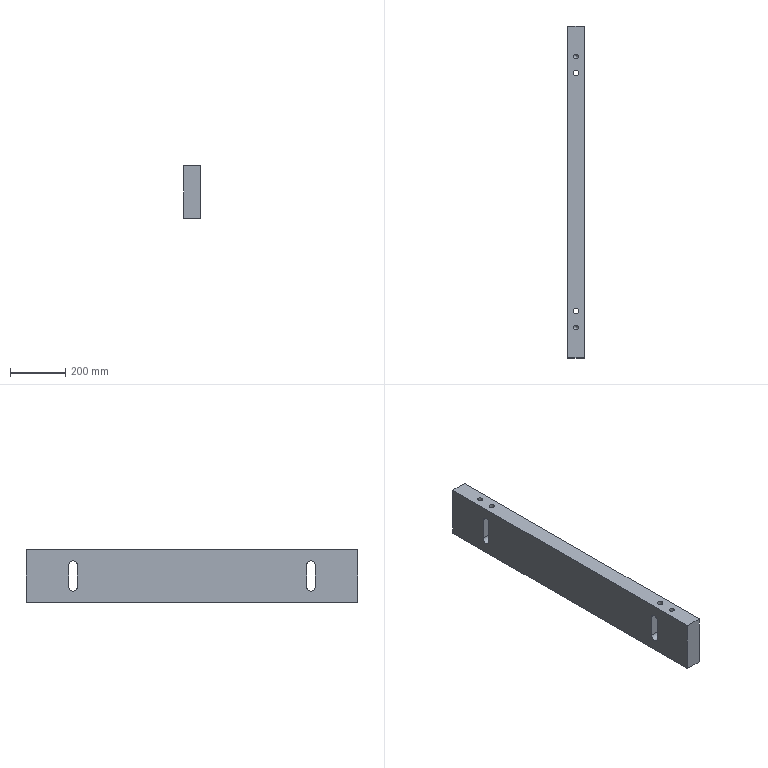Part | STEP file | lll_id4454_x_t | 1 solid | 30 faces | box 60 x 1200 x 190 mm | volume 13210878 mm3 | cylinder 14 | plane 10 | cone 6 | commonest cylinder face diameters 20 x4 30 x4 6.806 x2 17.505 x2 17.506 x2
STEP:
#1=CARTESIAN_POINT('',(207.435,-430.,-220.));
#2=VERTEX_POINT('',#1);
#3=CARTESIAN_POINT('',(207.435,-427.265,-220.));
#4=CARTESIAN_POINT('',(207.435,-432.735,-220.));
#5=CARTESIAN_POINT('',(206.282,-435.303,-220.824));
#6=CARTESIAN_POINT('',(203.596,-437.978,-222.257));
#7=CARTESIAN_POINT('',(202.537,-438.697,-222.762));
#8=CARTESIAN_POINT('',(200.161,-439.708,-223.547));
#9=CARTESIAN_POINT('',(198.811,-439.997,-223.817));
#10=CARTESIAN_POINT('',(194.742,-440.005,-223.824));
#11=CARTESIAN_POINT('',(192.2,-438.892,-222.75));
#12=CARTESIAN_POINT('',(189.491,-436.205,-221.306));
#13=CARTESIAN_POINT('',(188.758,-435.142,-220.853));
#14=CARTESIAN_POINT('',(187.723,-432.721,-220.196));
#15=CARTESIAN_POINT('',(187.438,-431.369,-220.002));
#16=CARTESIAN_POINT('',(187.432,-428.674,-219.998));
#17=CARTESIAN_POINT('',(187.71,-427.321,-220.187));
#18=CARTESIAN_POINT('',(188.743,-424.881,-220.844));
#19=CARTESIAN_POINT('',(189.483,-423.806,-221.301));
#20=CARTESIAN_POINT('',(192.176,-421.125,-222.738));
#21=CARTESIAN_POINT('',(194.698,-420.001,-223.819));
#22=CARTESIAN_POINT('',(200.165,-419.999,-223.821));
#23=CARTESIAN_POINT('',(202.693,-421.126,-222.738));
#24=CARTESIAN_POINT('',(206.281,-424.694,-220.824));
#25=CARTESIAN_POINT('',(207.435,-427.265,-220.));
#26=CARTESIAN_POINT('',(207.435,-432.735,-220.));
#27=B_SPLINE_CURVE_WITH_KNOTS('',3,(#3,#4,#5,#6,#7,#8,#9,#10,#11,#12,#13,#14,#15,#16,#17,#18,#19,#20,#21,#22,#23,#24,#25,#26),.UNSPECIFIED.,.T.,.F.,(2,2,2,2,2,2,2,2,2,2,2,2,2,2),(-0.125,0.,0.125,0.1875,0.25,0.375,0.4375,0.5,0.5625,0.625,0.75,0.875,1.,1.125),.UNSPECIFIED.);
#28=EDGE_CURVE('',#2,#2,#27,.T.);
#29=ORIENTED_EDGE('',*,*,#28,.T.);
#30=EDGE_LOOP('',(#29));
#31=FACE_BOUND('',#30,.T.);
#32=CARTESIAN_POINT('',(187.435,-430.,-180.));
#33=VERTEX_POINT('',#32);
#34=CARTESIAN_POINT('',(197.435,-430.,-180.));
#35=DIRECTION('',(0.,0.,-1.));
#36=DIRECTION('',(-1.,0.,0.));
#37=AXIS2_PLACEMENT_3D('',#34,#35,#36);
#38=CIRCLE('',#37,10.);
#39=EDGE_CURVE('',#33,#33,#38,.T.);
#40=ORIENTED_EDGE('',*,*,#39,.F.);
#41=EDGE_LOOP('',(#40));
#42=FACE_BOUND('',#41,.T.);
#43=CARTESIAN_POINT('',(197.435,-430.,-80.));
#44=DIRECTION('',(0.,0.,-1.));
#45=DIRECTION('',(-1.,0.,0.));
#46=AXIS2_PLACEMENT_3D('',#43,#44,#45);
#47=CYLINDRICAL_SURFACE('',#46,10.);
#48=ADVANCED_FACE('',(#31,#42),#47,.F.);
#49=CARTESIAN_POINT('',(207.435,430.,-220.));
#50=VERTEX_POINT('',#49);
#51=CARTESIAN_POINT('',(207.435,432.735,-220.));
#52=CARTESIAN_POINT('',(207.435,427.265,-220.));
#53=CARTESIAN_POINT('',(206.282,424.697,-220.824));
#54=CARTESIAN_POINT('',(203.596,422.022,-222.257));
#55=CARTESIAN_POINT('',(202.537,421.303,-222.762));
#56=CARTESIAN_POINT('',(200.161,420.292,-223.547));
#57=CARTESIAN_POINT('',(198.811,420.003,-223.817));
#58=CARTESIAN_POINT('',(194.742,419.995,-223.824));
#59=CARTESIAN_POINT('',(192.2,421.108,-222.75));
#60=CARTESIAN_POINT('',(189.491,423.795,-221.306));
#61=CARTESIAN_POINT('',(188.758,424.858,-220.853));
#62=CARTESIAN_POINT('',(187.723,427.279,-220.196));
#63=CARTESIAN_POINT('',(187.438,428.631,-220.002));
#64=CARTESIAN_POINT('',(187.432,431.326,-219.998));
#65=CARTESIAN_POINT('',(187.71,432.679,-220.187));
#66=CARTESIAN_POINT('',(188.743,435.119,-220.844));
#67=CARTESIAN_POINT('',(189.483,436.194,-221.301));
#68=CARTESIAN_POINT('',(192.176,438.875,-222.738));
#69=CARTESIAN_POINT('',(194.698,439.999,-223.819));
#70=CARTESIAN_POINT('',(200.165,440.001,-223.821));
#71=CARTESIAN_POINT('',(202.693,438.874,-222.738));
#72=CARTESIAN_POINT('',(206.281,435.306,-220.824));
#73=CARTESIAN_POINT('',(207.435,432.735,-220.));
#74=CARTESIAN_POINT('',(207.435,427.265,-220.));
#75=B_SPLINE_CURVE_WITH_KNOTS('',3,(#51,#52,#53,#54,#55,#56,#57,#58,#59,#60,#61,#62,#63,#64,#65,#66,#67,#68,#69,#70,#71,#72,#73,#74),.UNSPECIFIED.,.T.,.F.,(2,2,2,2,2,2,2,2,2,2,2,2,2,2),(-0.125,0.,0.125,0.1875,0.25,0.375,0.4375,0.5,0.5625,0.625,0.75,0.875,1.,1.125),.UNSPECIFIED.);
#76=EDGE_CURVE('',#50,#50,#75,.T.);
#77=ORIENTED_EDGE('',*,*,#76,.T.);
#78=EDGE_LOOP('',(#77));
#79=FACE_BOUND('',#78,.T.);
#80=CARTESIAN_POINT('',(187.435,430.,-180.));
#81=VERTEX_POINT('',#80);
#82=CARTESIAN_POINT('',(197.435,430.,-180.));
#83=DIRECTION('',(0.,0.,-1.));
#84=DIRECTION('',(-1.,0.,0.));
#85=AXIS2_PLACEMENT_3D('',#82,#83,#84);
#86=CIRCLE('',#85,10.);
#87=EDGE_CURVE('',#81,#81,#86,.T.);
#88=ORIENTED_EDGE('',*,*,#87,.F.);
#89=EDGE_LOOP('',(#88));
#90=FACE_BOUND('',#89,.T.);
#91=CARTESIAN_POINT('',(197.435,430.,-80.));
#92=DIRECTION('',(0.,0.,-1.));
#93=DIRECTION('',(-1.,0.,0.));
#94=AXIS2_PLACEMENT_3D('',#91,#92,#93);
#95=CYLINDRICAL_SURFACE('',#94,10.);
#96=ADVANCED_FACE('',(#79,#90),#95,.F.);
#97=CARTESIAN_POINT('',(227.435,-445.,-235.));
#98=VERTEX_POINT('',#97);
#99=CARTESIAN_POINT('',(227.435,-445.,-315.));
#100=VERTEX_POINT('',#99);
#101=CARTESIAN_POINT('',(227.435,-445.,-182.5));
#102=DIRECTION('',(0.,0.,-1.));
#103=VECTOR('',#102,1.);
#104=LINE('',#101,#103);
#105=EDGE_CURVE('',#98,#100,#104,.T.);
#106=ORIENTED_EDGE('',*,*,#105,.F.);
#107=CARTESIAN_POINT('',(227.435,-415.,-235.));
#108=VERTEX_POINT('',#107);
#109=CARTESIAN_POINT('',(227.435,-430.,-235.));
#110=DIRECTION('',(1.,0.,0.));
#111=DIRECTION('',(0.,0.,-1.));
#112=AXIS2_PLACEMENT_3D('',#109,#110,#111);
#113=CIRCLE('',#112,15.);
#114=EDGE_CURVE('',#108,#98,#113,.T.);
#115=ORIENTED_EDGE('',*,*,#114,.F.);
#116=CARTESIAN_POINT('',(227.435,-415.,-315.));
#117=VERTEX_POINT('',#116);
#118=CARTESIAN_POINT('',(227.435,-415.,-182.5));
#119=DIRECTION('',(0.,0.,1.));
#120=VECTOR('',#119,1.);
#121=LINE('',#118,#120);
#122=EDGE_CURVE('',#117,#108,#121,.T.);
#123=ORIENTED_EDGE('',*,*,#122,.F.);
#124=CARTESIAN_POINT('',(227.435,-430.,-315.));
#125=DIRECTION('',(1.,0.,0.));
#126=DIRECTION('',(0.,0.,-1.));
#127=AXIS2_PLACEMENT_3D('',#124,#125,#126);
#128=CIRCLE('',#127,15.);
#129=EDGE_CURVE('',#100,#117,#128,.T.);
#130=ORIENTED_EDGE('',*,*,#129,.F.);
#131=EDGE_LOOP('',(#106,#115,#123,#130));
#132=FACE_BOUND('',#131,.T.);
#133=CARTESIAN_POINT('',(227.435,415.,-235.));
#134=VERTEX_POINT('',#133);
#135=CARTESIAN_POINT('',(227.435,415.,-315.));
#136=VERTEX_POINT('',#135);
#137=CARTESIAN_POINT('',(227.435,415.,-182.5));
#138=DIRECTION('',(0.,0.,-1.));
#139=VECTOR('',#138,1.);
#140=LINE('',#137,#139);
#141=EDGE_CURVE('',#134,#136,#140,.T.);
#142=ORIENTED_EDGE('',*,*,#141,.F.);
#143=CARTESIAN_POINT('',(227.435,445.,-235.));
#144=VERTEX_POINT('',#143);
#145=CARTESIAN_POINT('',(227.435,430.,-235.));
#146=DIRECTION('',(1.,0.,0.));
#147=DIRECTION('',(0.,0.,-1.));
#148=AXIS2_PLACEMENT_3D('',#145,#146,#147);
#149=CIRCLE('',#148,15.);
#150=EDGE_CURVE('',#144,#134,#149,.T.);
#151=ORIENTED_EDGE('',*,*,#150,.F.);
#152=CARTESIAN_POINT('',(227.435,445.,-315.));
#153=VERTEX_POINT('',#152);
#154=CARTESIAN_POINT('',(227.435,445.,-182.5));
#155=DIRECTION('',(0.,0.,1.));
#156=VECTOR('',#155,1.);
#157=LINE('',#154,#156);
#158=EDGE_CURVE('',#153,#144,#157,.T.);
#159=ORIENTED_EDGE('',*,*,#158,.F.);
#160=CARTESIAN_POINT('',(227.435,430.,-315.));
#161=DIRECTION('',(1.,0.,0.));
#162=DIRECTION('',(0.,0.,-1.));
#163=AXIS2_PLACEMENT_3D('',#160,#161,#162);
#164=CIRCLE('',#163,15.);
#165=EDGE_CURVE('',#136,#153,#164,.T.);
#166=ORIENTED_EDGE('',*,*,#165,.F.);
#167=EDGE_LOOP('',(#142,#151,#159,#166));
#168=FACE_BOUND('',#167,.T.);
#169=CARTESIAN_POINT('',(227.435,109.597,-194.345));
#170=VERTEX_POINT('',#169);
#171=CARTESIAN_POINT('',(227.435,113.,-194.345));
#172=DIRECTION('',(-1.,0.,0.));
#173=DIRECTION('',(0.,-1.,0.));
#174=AXIS2_PLACEMENT_3D('',#171,#172,#173);
#175=CIRCLE('',#174,3.403);
#176=EDGE_CURVE('',#170,#170,#175,.T.);
#177=ORIENTED_EDGE('',*,*,#176,.T.);
#178=EDGE_LOOP('',(#177));
#179=FACE_BOUND('',#178,.T.);
#180=CARTESIAN_POINT('',(227.435,-600.,-180.));
#181=VERTEX_POINT('',#180);
#182=CARTESIAN_POINT('',(227.435,-600.,-370.));
#183=VERTEX_POINT('',#182);
#184=CARTESIAN_POINT('',(227.435,-600.,-182.5));
#185=DIRECTION('',(0.,0.,-1.));
#186=VECTOR('',#185,1.);
#187=LINE('',#184,#186);
#188=EDGE_CURVE('',#181,#183,#187,.T.);
#189=ORIENTED_EDGE('',*,*,#188,.T.);
#190=CARTESIAN_POINT('',(227.435,600.,-370.));
#191=VERTEX_POINT('',#190);
#192=CARTESIAN_POINT('',(227.435,600.,-370.));
#193=DIRECTION('',(0.,-1.,0.));
#194=VECTOR('',#193,1.);
#195=LINE('',#192,#194);
#196=EDGE_CURVE('',#191,#183,#195,.T.);
#197=ORIENTED_EDGE('',*,*,#196,.F.);
#198=CARTESIAN_POINT('',(227.435,600.,-180.));
#199=VERTEX_POINT('',#198);
#200=CARTESIAN_POINT('',(227.435,600.,-182.5));
#201=DIRECTION('',(0.,0.,-1.));
#202=VECTOR('',#201,1.);
#203=LINE('',#200,#202);
#204=EDGE_CURVE('',#199,#191,#203,.T.);
#205=ORIENTED_EDGE('',*,*,#204,.F.);
#206=CARTESIAN_POINT('',(227.435,1.,-180.));
#207=DIRECTION('',(0.,-1.,0.));
#208=VECTOR('',#207,1.);
#209=LINE('',#206,#208);
#210=EDGE_CURVE('',#199,#181,#209,.T.);
#211=ORIENTED_EDGE('',*,*,#210,.T.);
#212=EDGE_LOOP('',(#189,#197,#205,#211));
#213=FACE_BOUND('',#212,.T.);
#214=CARTESIAN_POINT('',(227.435,-206.403,-194.345));
#215=VERTEX_POINT('',#214);
#216=CARTESIAN_POINT('',(227.435,-203.,-194.345));
#217=DIRECTION('',(-1.,0.,0.));
#218=DIRECTION('',(0.,-1.,0.));
#219=AXIS2_PLACEMENT_3D('',#216,#217,#218);
#220=CIRCLE('',#219,3.403);
#221=EDGE_CURVE('',#215,#215,#220,.T.);
#222=ORIENTED_EDGE('',*,*,#221,.T.);
#223=EDGE_LOOP('',(#222));
#224=FACE_BOUND('',#223,.T.);
#225=CARTESIAN_POINT('',(227.435,600.,-182.5));
#226=DIRECTION('',(1.,0.,0.));
#227=DIRECTION('',(0.,0.,-1.));
#228=AXIS2_PLACEMENT_3D('',#225,#226,#227);
#229=PLANE('',#228);
#230=ADVANCED_FACE('',(#132,#168,#179,#213,#224),#229,.T.);
#231=CARTESIAN_POINT('',(187.435,430.,-370.));
#232=VERTEX_POINT('',#231);
#233=CARTESIAN_POINT('',(197.435,430.,-370.));
#234=DIRECTION('',(0.,0.,-1.));
#235=DIRECTION('',(-1.,0.,0.));
#236=AXIS2_PLACEMENT_3D('',#233,#234,#235);
#237=CIRCLE('',#236,10.);
#238=EDGE_CURVE('',#232,#232,#237,.T.);
#239=ORIENTED_EDGE('',*,*,#238,.F.);
#240=EDGE_LOOP('',(#239));
#241=FACE_BOUND('',#240,.T.);
#242=CARTESIAN_POINT('',(187.435,-430.,-370.));
#243=VERTEX_POINT('',#242);
#244=CARTESIAN_POINT('',(197.435,-430.,-370.));
#245=DIRECTION('',(0.,0.,-1.));
#246=DIRECTION('',(-1.,0.,0.));
#247=AXIS2_PLACEMENT_3D('',#244,#245,#246);
#248=CIRCLE('',#247,10.);
#249=EDGE_CURVE('',#243,#243,#248,.T.);
#250=ORIENTED_EDGE('',*,*,#249,.F.);
#251=EDGE_LOOP('',(#250));
#252=FACE_BOUND('',#251,.T.);
#253=CARTESIAN_POINT('',(206.188,-490.,-370.));
#254=VERTEX_POINT('',#253);
#255=CARTESIAN_POINT('',(197.435,-490.,-370.));
#256=DIRECTION('',(0.,0.,1.));
#257=DIRECTION('',(1.,0.,0.));
#258=AXIS2_PLACEMENT_3D('',#255,#256,#257);
#259=CIRCLE('',#258,8.752);
#260=EDGE_CURVE('',#254,#254,#259,.T.);
#261=ORIENTED_EDGE('',*,*,#260,.T.);
#262=EDGE_LOOP('',(#261));
#263=FACE_BOUND('',#262,.T.);
#264=ORIENTED_EDGE('',*,*,#196,.T.);
#265=CARTESIAN_POINT('',(167.435,-600.,-370.));
#266=VERTEX_POINT('',#265);
#267=CARTESIAN_POINT('',(227.435,-600.,-370.));
#268=DIRECTION('',(-1.,0.,0.));
#269=VECTOR('',#268,1.);
#270=LINE('',#267,#269);
#271=EDGE_CURVE('',#183,#266,#270,.T.);
#272=ORIENTED_EDGE('',*,*,#271,.T.);
#273=CARTESIAN_POINT('',(167.435,600.,-370.));
#274=VERTEX_POINT('',#273);
#275=CARTESIAN_POINT('',(167.435,1.,-370.));
#276=DIRECTION('',(0.,-1.,0.));
#277=VECTOR('',#276,1.);
#278=LINE('',#275,#277);
#279=EDGE_CURVE('',#274,#266,#278,.T.);
#280=ORIENTED_EDGE('',*,*,#279,.F.);
#281=CARTESIAN_POINT('',(-3742.565,600.,-370.));
#282=DIRECTION('',(1.,0.,0.));
#283=VECTOR('',#282,1.);
#284=LINE('',#281,#283);
#285=EDGE_CURVE('',#274,#191,#284,.T.);
#286=ORIENTED_EDGE('',*,*,#285,.T.);
#287=EDGE_LOOP('',(#264,#272,#280,#286));
#288=FACE_BOUND('',#287,.T.);
#289=CARTESIAN_POINT('',(206.188,490.,-370.));
#290=VERTEX_POINT('',#289);
#291=CARTESIAN_POINT('',(197.435,490.,-370.));
#292=DIRECTION('',(0.,0.,1.));
#293=DIRECTION('',(1.,0.,0.));
#294=AXIS2_PLACEMENT_3D('',#291,#292,#293);
#295=CIRCLE('',#294,8.752);
#296=EDGE_CURVE('',#290,#290,#295,.T.);
#297=ORIENTED_EDGE('',*,*,#296,.T.);
#298=EDGE_LOOP('',(#297));
#299=FACE_BOUND('',#298,.T.);
#300=CARTESIAN_POINT('',(2413.751,1.,-370.));
#301=DIRECTION('',(0.,0.,-1.));
#302=DIRECTION('',(-1.,0.,0.));
#303=AXIS2_PLACEMENT_3D('',#300,#301,#302);
#304=PLANE('',#303);
#305=ADVANCED_FACE('',(#241,#252,#263,#288,#299),#304,.T.);
#306=ORIENTED_EDGE('',*,*,#39,.T.);
#307=EDGE_LOOP('',(#306));
#308=FACE_BOUND('',#307,.T.);
#309=ORIENTED_EDGE('',*,*,#87,.T.);
#310=EDGE_LOOP('',(#309));
#311=FACE_BOUND('',#310,.T.);
#312=CARTESIAN_POINT('',(188.682,490.,-180.));
#313=VERTEX_POINT('',#312);
#314=CARTESIAN_POINT('',(197.435,490.,-180.));
#315=DIRECTION('',(0.,0.,-1.));
#316=DIRECTION('',(-1.,0.,0.));
#317=AXIS2_PLACEMENT_3D('',#314,#315,#316);
#318=CIRCLE('',#317,8.753);
#319=EDGE_CURVE('',#313,#313,#318,.T.);
#320=ORIENTED_EDGE('',*,*,#319,.T.);
#321=EDGE_LOOP('',(#320));
#322=FACE_BOUND('',#321,.T.);
#323=CARTESIAN_POINT('',(188.682,-490.,-180.));
#324=VERTEX_POINT('',#323);
#325=CARTESIAN_POINT('',(197.435,-490.,-180.));
#326=DIRECTION('',(0.,0.,-1.));
#327=DIRECTION('',(-1.,0.,0.));
#328=AXIS2_PLACEMENT_3D('',#325,#326,#327);
#329=CIRCLE('',#328,8.753);
#330=EDGE_CURVE('',#324,#324,#329,.T.);
#331=ORIENTED_EDGE('',*,*,#330,.T.);
#332=EDGE_LOOP('',(#331));
#333=FACE_BOUND('',#332,.T.);
#334=CARTESIAN_POINT('',(167.435,-600.,-180.));
#335=VERTEX_POINT('',#334);
#336=CARTESIAN_POINT('',(2413.751,-600.,-180.));
#337=DIRECTION('',(-1.,0.,0.));
#338=VECTOR('',#337,1.);
#339=LINE('',#336,#338);
#340=EDGE_CURVE('',#181,#335,#339,.T.);
#341=ORIENTED_EDGE('',*,*,#340,.F.);
#342=ORIENTED_EDGE('',*,*,#210,.F.);
#343=CARTESIAN_POINT('',(167.435,600.,-180.));
#344=VERTEX_POINT('',#343);
#345=CARTESIAN_POINT('',(2413.751,600.,-180.));
#346=DIRECTION('',(1.,0.,0.));
#347=VECTOR('',#346,1.);
#348=LINE('',#345,#347);
#349=EDGE_CURVE('',#344,#199,#348,.T.);
#350=ORIENTED_EDGE('',*,*,#349,.F.);
#351=CARTESIAN_POINT('',(167.435,0.,-180.));
#352=DIRECTION('',(0.,1.,0.));
#353=VECTOR('',#352,1.);
#354=LINE('',#351,#353);
#355=EDGE_CURVE('',#335,#344,#354,.T.);
#356=ORIENTED_EDGE('',*,*,#355,.F.);
#357=EDGE_LOOP('',(#341,#342,#350,#356));
#358=FACE_BOUND('',#357,.T.);
#359=CARTESIAN_POINT('',(2413.751,1.,-180.));
#360=DIRECTION('',(0.,0.,-1.));
#361=DIRECTION('',(-1.,0.,0.));
#362=AXIS2_PLACEMENT_3D('',#359,#360,#361);
#363=PLANE('',#362);
#364=ADVANCED_FACE('',(#308,#311,#322,#333,#358),#363,.F.);
#365=CARTESIAN_POINT('',(167.435,-600.,-182.5));
#366=DIRECTION('',(0.,0.,-1.));
#367=VECTOR('',#366,1.);
#368=LINE('',#365,#367);
#369=EDGE_CURVE('',#335,#266,#368,.T.);
#370=ORIENTED_EDGE('',*,*,#369,.T.);
#371=ORIENTED_EDGE('',*,*,#271,.F.);
#372=ORIENTED_EDGE('',*,*,#188,.F.);
#373=ORIENTED_EDGE('',*,*,#340,.T.);
#374=EDGE_LOOP('',(#370,#371,#372,#373));
#375=FACE_OUTER_BOUND('',#374,.T.);
#376=CARTESIAN_POINT('',(227.435,-600.,-182.5));
#377=DIRECTION('',(0.,-1.,0.));
#378=DIRECTION('',(0.,0.,-1.));
#379=AXIS2_PLACEMENT_3D('',#376,#377,#378);
#380=PLANE('',#379);
#381=ADVANCED_FACE('',(#375),#380,.T.);
#382=CARTESIAN_POINT('',(167.435,600.,-182.5));
#383=DIRECTION('',(0.,0.,1.));
#384=VECTOR('',#383,1.);
#385=LINE('',#382,#384);
#386=EDGE_CURVE('',#274,#344,#385,.T.);
#387=ORIENTED_EDGE('',*,*,#386,.T.);
#388=ORIENTED_EDGE('',*,*,#349,.T.);
#389=ORIENTED_EDGE('',*,*,#204,.T.);
#390=ORIENTED_EDGE('',*,*,#285,.F.);
#391=EDGE_LOOP('',(#387,#388,#389,#390));
#392=FACE_OUTER_BOUND('',#391,.T.);
#393=CARTESIAN_POINT('',(-3742.565,600.,-182.5));
#394=DIRECTION('',(0.,1.,0.));
#395=DIRECTION('',(0.,0.,1.));
#396=AXIS2_PLACEMENT_3D('',#393,#394,#395);
#397=PLANE('',#396);
#398=ADVANCED_FACE('',(#392),#397,.T.);
#399=CARTESIAN_POINT('',(167.435,-415.,-235.));
#400=VERTEX_POINT('',#399);
#401=CARTESIAN_POINT('',(167.435,-445.,-235.));
#402=VERTEX_POINT('',#401);
#403=CARTESIAN_POINT('',(167.435,-430.,-235.));
#404=DIRECTION('',(1.,0.,0.));
#405=DIRECTION('',(0.,0.,-1.));
#406=AXIS2_PLACEMENT_3D('',#403,#404,#405);
#407=CIRCLE('',#406,15.);
#408=EDGE_CURVE('',#400,#402,#407,.T.);
#409=ORIENTED_EDGE('',*,*,#408,.T.);
#410=CARTESIAN_POINT('',(167.435,-445.,-315.));
#411=VERTEX_POINT('',#410);
#412=CARTESIAN_POINT('',(167.435,-445.,-251.25));
#413=DIRECTION('',(0.,0.,-1.));
#414=VECTOR('',#413,1.);
#415=LINE('',#412,#414);
#416=EDGE_CURVE('',#402,#411,#415,.T.);
#417=ORIENTED_EDGE('',*,*,#416,.T.);
#418=CARTESIAN_POINT('',(167.435,-415.,-315.));
#419=VERTEX_POINT('',#418);
#420=CARTESIAN_POINT('',(167.435,-430.,-315.));
#421=DIRECTION('',(1.,0.,0.));
#422=DIRECTION('',(0.,0.,-1.));
#423=AXIS2_PLACEMENT_3D('',#420,#421,#422);
#424=CIRCLE('',#423,15.);
#425=EDGE_CURVE('',#411,#419,#424,.T.);
#426=ORIENTED_EDGE('',*,*,#425,.T.);
#427=CARTESIAN_POINT('',(167.435,-415.,-251.25));
#428=DIRECTION('',(0.,0.,1.));
#429=VECTOR('',#428,1.);
#430=LINE('',#427,#429);
#431=EDGE_CURVE('',#419,#400,#430,.T.);
#432=ORIENTED_EDGE('',*,*,#431,.T.);
#433=EDGE_LOOP('',(#409,#417,#426,#432));
#434=FACE_BOUND('',#433,.T.);
#435=CARTESIAN_POINT('',(167.435,445.,-235.));
#436=VERTEX_POINT('',#435);
#437=CARTESIAN_POINT('',(167.435,415.,-235.));
#438=VERTEX_POINT('',#437);
#439=CARTESIAN_POINT('',(167.435,430.,-235.));
#440=DIRECTION('',(1.,0.,0.));
#441=DIRECTION('',(0.,0.,-1.));
#442=AXIS2_PLACEMENT_3D('',#439,#440,#441);
#443=CIRCLE('',#442,15.);
#444=EDGE_CURVE('',#436,#438,#443,.T.);
#445=ORIENTED_EDGE('',*,*,#444,.T.);
#446=CARTESIAN_POINT('',(167.435,415.,-315.));
#447=VERTEX_POINT('',#446);
#448=CARTESIAN_POINT('',(167.435,415.,-251.25));
#449=DIRECTION('',(0.,0.,-1.));
#450=VECTOR('',#449,1.);
#451=LINE('',#448,#450);
#452=EDGE_CURVE('',#438,#447,#451,.T.);
#453=ORIENTED_EDGE('',*,*,#452,.T.);
#454=CARTESIAN_POINT('',(167.435,445.,-315.));
#455=VERTEX_POINT('',#454);
#456=CARTESIAN_POINT('',(167.435,430.,-315.));
#457=DIRECTION('',(1.,0.,0.));
#458=DIRECTION('',(0.,0.,-1.));
#459=AXIS2_PLACEMENT_3D('',#456,#457,#458);
#460=CIRCLE('',#459,15.);
#461=EDGE_CURVE('',#447,#455,#460,.T.);
#462=ORIENTED_EDGE('',*,*,#461,.T.);
#463=CARTESIAN_POINT('',(167.435,445.,-251.25));
#464=DIRECTION('',(0.,0.,1.));
#465=VECTOR('',#464,1.);
#466=LINE('',#463,#465);
#467=EDGE_CURVE('',#455,#436,#466,.T.);
#468=ORIENTED_EDGE('',*,*,#467,.T.);
#469=EDGE_LOOP('',(#445,#453,#462,#468));
#470=FACE_BOUND('',#469,.T.);
#471=ORIENTED_EDGE('',*,*,#386,.F.);
#472=ORIENTED_EDGE('',*,*,#279,.T.);
#473=ORIENTED_EDGE('',*,*,#369,.F.);
#474=ORIENTED_EDGE('',*,*,#355,.T.);
#475=EDGE_LOOP('',(#471,#472,#473,#474));
#476=FACE_BOUND('',#475,.T.);
#477=CARTESIAN_POINT('',(167.435,0.,-251.25));
#478=DIRECTION('',(1.,0.,0.));
#479=DIRECTION('',(0.,0.,-1.));
#480=AXIS2_PLACEMENT_3D('',#477,#478,#479);
#481=PLANE('',#480);
#482=ADVANCED_FACE('',(#434,#470,#476),#481,.F.);
#483=CARTESIAN_POINT('',(206.188,-490.,-328.747));
#484=VERTEX_POINT('',#483);
#485=CARTESIAN_POINT('',(197.435,-490.,-328.747));
#486=DIRECTION('',(0.,0.,1.));
#487=DIRECTION('',(1.,0.,0.));
#488=AXIS2_PLACEMENT_3D('',#485,#486,#487);
#489=CIRCLE('',#488,8.752);
#490=EDGE_CURVE('',#484,#484,#489,.T.);
#491=ORIENTED_EDGE('',*,*,#490,.T.);
#492=EDGE_LOOP('',(#491));
#493=FACE_BOUND('',#492,.T.);
#494=ORIENTED_EDGE('',*,*,#260,.F.);
#495=EDGE_LOOP('',(#494));
#496=FACE_BOUND('',#495,.T.);
#497=CARTESIAN_POINT('',(197.435,-490.,-370.));
#498=DIRECTION('',(0.,0.,1.));
#499=DIRECTION('',(-1.,0.,0.));
#500=AXIS2_PLACEMENT_3D('',#497,#498,#499);
#501=CYLINDRICAL_SURFACE('',#500,8.752);
#502=ADVANCED_FACE('',(#493,#496),#501,.F.);
#503=CARTESIAN_POINT('',(197.435,-490.,-319.994));
#504=VERTEX_POINT('',#503);
#505=VERTEX_LOOP('',#504);
#506=FACE_BOUND('',#505,.T.);
#507=ORIENTED_EDGE('',*,*,#490,.F.);
#508=EDGE_LOOP('',(#507));
#509=FACE_BOUND('',#508,.T.);
#510=CARTESIAN_POINT('',(197.435,-490.,-328.747));
#511=DIRECTION('',(0.,0.,-1.));
#512=DIRECTION('',(1.,0.,0.));
#513=AXIS2_PLACEMENT_3D('',#510,#511,#512);
#514=CONICAL_SURFACE('',#513,8.752,45.);
#515=ADVANCED_FACE('',(#506,#509),#514,.F.);
#516=CARTESIAN_POINT('',(206.188,490.,-328.747));
#517=VERTEX_POINT('',#516);
#518=CARTESIAN_POINT('',(197.435,490.,-328.747));
#519=DIRECTION('',(0.,0.,1.));
#520=DIRECTION('',(1.,0.,0.));
#521=AXIS2_PLACEMENT_3D('',#518,#519,#520);
#522=CIRCLE('',#521,8.752);
#523=EDGE_CURVE('',#517,#517,#522,.T.);
#524=ORIENTED_EDGE('',*,*,#523,.T.);
#525=EDGE_LOOP('',(#524));
#526=FACE_BOUND('',#525,.T.);
#527=ORIENTED_EDGE('',*,*,#296,.F.);
#528=EDGE_LOOP('',(#527));
#529=FACE_BOUND('',#528,.T.);
#530=CARTESIAN_POINT('',(197.435,490.,-370.));
#531=DIRECTION('',(0.,0.,1.));
#532=DIRECTION('',(-1.,0.,0.));
#533=AXIS2_PLACEMENT_3D('',#530,#531,#532);
#534=CYLINDRICAL_SURFACE('',#533,8.752);
#535=ADVANCED_FACE('',(#526,#529),#534,.F.);
#536=CARTESIAN_POINT('',(197.435,490.,-319.994));
#537=VERTEX_POINT('',#536);
#538=VERTEX_LOOP('',#537);
#539=FACE_BOUND('',#538,.T.);
#540=ORIENTED_EDGE('',*,*,#523,.F.);
#541=EDGE_LOOP('',(#540));
#542=FACE_BOUND('',#541,.T.);
#543=CARTESIAN_POINT('',(197.435,490.,-328.747));
#544=DIRECTION('',(0.,0.,-1.));
#545=DIRECTION('',(1.,0.,0.));
#546=AXIS2_PLACEMENT_3D('',#543,#544,#545);
#547=CONICAL_SURFACE('',#546,8.752,45.);
#548=ADVANCED_FACE('',(#539,#542),#547,.F.);
#549=CARTESIAN_POINT('',(188.682,-490.,-221.253));
#550=VERTEX_POINT('',#549);
#551=CARTESIAN_POINT('',(197.435,-490.,-221.253));
#552=DIRECTION('',(0.,0.,-1.));
#553=DIRECTION('',(-1.,0.,0.));
#554=AXIS2_PLACEMENT_3D('',#551,#552,#553);
#555=CIRCLE('',#554,8.753);
#556=EDGE_CURVE('',#550,#550,#555,.T.);
#557=ORIENTED_EDGE('',*,*,#556,.T.);
#558=EDGE_LOOP('',(#557));
#559=FACE_BOUND('',#558,.T.);
#560=ORIENTED_EDGE('',*,*,#330,.F.);
#561=EDGE_LOOP('',(#560));
#562=FACE_BOUND('',#561,.T.);
#563=CARTESIAN_POINT('',(197.435,-490.,-180.));
#564=DIRECTION('',(0.,0.,-1.));
#565=DIRECTION('',(1.,0.,0.));
#566=AXIS2_PLACEMENT_3D('',#563,#564,#565);
#567=CYLINDRICAL_SURFACE('',#566,8.753);
#568=ADVANCED_FACE('',(#559,#562),#567,.F.);
#569=CARTESIAN_POINT('',(197.435,-490.,-230.006));
#570=VERTEX_POINT('',#569);
#571=VERTEX_LOOP('',#570);
#572=FACE_BOUND('',#571,.T.);
#573=ORIENTED_EDGE('',*,*,#556,.F.);
#574=EDGE_LOOP('',(#573));
#575=FACE_BOUND('',#574,.T.);
#576=CARTESIAN_POINT('',(197.435,-490.,-221.253));
#577=DIRECTION('',(0.,0.,1.));
#578=DIRECTION('',(-1.,0.,0.));
#579=AXIS2_PLACEMENT_3D('',#576,#577,#578);
#580=CONICAL_SURFACE('',#579,8.753,45.);
#581=ADVANCED_FACE('',(#572,#575),#580,.F.);
#582=CARTESIAN_POINT('',(188.682,490.,-221.253));
#583=VERTEX_POINT('',#582);
#584=CARTESIAN_POINT('',(197.435,490.,-221.253));
#585=DIRECTION('',(0.,0.,-1.));
#586=DIRECTION('',(-1.,0.,0.));
#587=AXIS2_PLACEMENT_3D('',#584,#585,#586);
#588=CIRCLE('',#587,8.753);
#589=EDGE_CURVE('',#583,#583,#588,.T.);
#590=ORIENTED_EDGE('',*,*,#589,.T.);
#591=EDGE_LOOP('',(#590));
#592=FACE_BOUND('',#591,.T.);
#593=ORIENTED_EDGE('',*,*,#319,.F.);
#594=EDGE_LOOP('',(#593));
#595=FACE_BOUND('',#594,.T.);
#596=CARTESIAN_POINT('',(197.435,490.,-180.));
#597=DIRECTION('',(0.,0.,-1.));
#598=DIRECTION('',(1.,0.,0.));
#599=AXIS2_PLACEMENT_3D('',#596,#597,#598);
#600=CYLINDRICAL_SURFACE('',#599,8.753);
#601=ADVANCED_FACE('',(#592,#595),#600,.F.);
#602=CARTESIAN_POINT('',(197.435,490.,-230.006));
#603=VERTEX_POINT('',#602);
#604=VERTEX_LOOP('',#603);
#605=FACE_BOUND('',#604,.T.);
#606=ORIENTED_EDGE('',*,*,#589,.F.);
#607=EDGE_LOOP('',(#606));
#608=FACE_BOUND('',#607,.T.);
#609=CARTESIAN_POINT('',(197.435,490.,-221.253));
#610=DIRECTION('',(0.,0.,1.));
#611=DIRECTION('',(-1.,0.,0.));
#612=AXIS2_PLACEMENT_3D('',#609,#610,#611);
#613=CONICAL_SURFACE('',#612,8.753,45.);
#614=ADVANCED_FACE('',(#605,#608),#613,.F.);
#615=CARTESIAN_POINT('',(195.832,113.,-190.942));
#616=VERTEX_POINT('',#615);
#617=CARTESIAN_POINT('',(195.832,113.,-194.345));
#618=DIRECTION('',(-1.,0.,0.));
#619=DIRECTION('',(0.,0.,1.));
#620=AXIS2_PLACEMENT_3D('',#617,#618,#619);
#621=CIRCLE('',#620,3.403);
#622=EDGE_CURVE('',#616,#616,#621,.T.);
#623=ORIENTED_EDGE('',*,*,#622,.T.);
#624=EDGE_LOOP('',(#623));
#625=FACE_BOUND('',#624,.T.);
#626=ORIENTED_EDGE('',*,*,#176,.F.);
#627=EDGE_LOOP('',(#626));
#628=FACE_BOUND('',#627,.T.);
#629=CARTESIAN_POINT('',(227.435,113.,-194.345));
#630=DIRECTION('',(-1.,0.,0.));
#631=DIRECTION('',(0.,1.,0.));
#632=AXIS2_PLACEMENT_3D('',#629,#630,#631);
#633=CYLINDRICAL_SURFACE('',#632,3.403);
#634=ADVANCED_FACE('',(#625,#628),#633,.F.);
#635=CARTESIAN_POINT('',(192.429,113.,-194.345));
#636=VERTEX_POINT('',#635);
#637=VERTEX_LOOP('',#636);
#638=FACE_BOUND('',#637,.T.);
#639=ORIENTED_EDGE('',*,*,#622,.F.);
#640=EDGE_LOOP('',(#639));
#641=FACE_BOUND('',#640,.T.);
#642=CARTESIAN_POINT('',(195.832,113.,-194.345));
#643=DIRECTION('',(1.,0.,0.));
#644=DIRECTION('',(0.,0.,1.));
#645=AXIS2_PLACEMENT_3D('',#642,#643,#644);
#646=CONICAL_SURFACE('',#645,3.403,45.);
#647=ADVANCED_FACE('',(#638,#641),#646,.F.);
#648=CARTESIAN_POINT('',(195.832,-203.,-190.942));
#649=VERTEX_POINT('',#648);
#650=CARTESIAN_POINT('',(195.832,-203.,-194.345));
#651=DIRECTION('',(-1.,0.,0.));
#652=DIRECTION('',(0.,0.,1.));
#653=AXIS2_PLACEMENT_3D('',#650,#651,#652);
#654=CIRCLE('',#653,3.403);
#655=EDGE_CURVE('',#649,#649,#654,.T.);
#656=ORIENTED_EDGE('',*,*,#655,.T.);
#657=EDGE_LOOP('',(#656));
#658=FACE_BOUND('',#657,.T.);
#659=ORIENTED_EDGE('',*,*,#221,.F.);
#660=EDGE_LOOP('',(#659));
#661=FACE_BOUND('',#660,.T.);
#662=CARTESIAN_POINT('',(227.435,-203.,-194.345));
#663=DIRECTION('',(-1.,0.,0.));
#664=DIRECTION('',(0.,1.,0.));
#665=AXIS2_PLACEMENT_3D('',#662,#663,#664);
#666=CYLINDRICAL_SURFACE('',#665,3.403);
#667=ADVANCED_FACE('',(#658,#661),#666,.F.);
#668=CARTESIAN_POINT('',(192.429,-203.,-194.345));
#669=VERTEX_POINT('',#668);
#670=VERTEX_LOOP('',#669);
#671=FACE_BOUND('',#670,.T.);
#672=ORIENTED_EDGE('',*,*,#655,.F.);
#673=EDGE_LOOP('',(#672));
#674=FACE_BOUND('',#673,.T.);
#675=CARTESIAN_POINT('',(195.832,-203.,-194.345));
#676=DIRECTION('',(1.,0.,0.));
#677=DIRECTION('',(0.,0.,1.));
#678=AXIS2_PLACEMENT_3D('',#675,#676,#677);
#679=CONICAL_SURFACE('',#678,3.403,45.);
#680=ADVANCED_FACE('',(#671,#674),#679,.F.);
#681=CARTESIAN_POINT('',(207.435,430.,-330.));
#682=VERTEX_POINT('',#681);
#683=CARTESIAN_POINT('',(207.435,427.265,-330.));
#684=CARTESIAN_POINT('',(207.435,432.735,-330.));
#685=CARTESIAN_POINT('',(206.282,435.303,-329.176));
#686=CARTESIAN_POINT('',(203.596,437.978,-327.743));
#687=CARTESIAN_POINT('',(202.537,438.697,-327.238));
#688=CARTESIAN_POINT('',(200.161,439.708,-326.453));
#689=CARTESIAN_POINT('',(198.811,439.997,-326.183));
#690=CARTESIAN_POINT('',(194.742,440.005,-326.176));
#691=CARTESIAN_POINT('',(192.2,438.892,-327.25));
#692=CARTESIAN_POINT('',(189.491,436.205,-328.694));
#693=CARTESIAN_POINT('',(188.758,435.142,-329.147));
#694=CARTESIAN_POINT('',(187.723,432.721,-329.804));
#695=CARTESIAN_POINT('',(187.438,431.369,-329.998));
#696=CARTESIAN_POINT('',(187.432,428.674,-330.002));
#697=CARTESIAN_POINT('',(187.71,427.321,-329.813));
#698=CARTESIAN_POINT('',(188.743,424.881,-329.156));
#699=CARTESIAN_POINT('',(189.483,423.806,-328.699));
#700=CARTESIAN_POINT('',(192.176,421.125,-327.262));
#701=CARTESIAN_POINT('',(194.698,420.001,-326.181));
#702=CARTESIAN_POINT('',(200.165,419.999,-326.179));
#703=CARTESIAN_POINT('',(202.693,421.126,-327.262));
#704=CARTESIAN_POINT('',(206.281,424.694,-329.176));
#705=CARTESIAN_POINT('',(207.435,427.265,-330.));
#706=CARTESIAN_POINT('',(207.435,432.735,-330.));
#707=B_SPLINE_CURVE_WITH_KNOTS('',3,(#683,#684,#685,#686,#687,#688,#689,#690,#691,#692,#693,#694,#695,#696,#697,#698,#699,#700,#701,#702,#703,#704,#705,#706),.UNSPECIFIED.,.T.,.F.,(2,2,2,2,2,2,2,2,2,2,2,2,2,2),(-0.125,0.,0.125,0.1875,0.25,0.375,0.4375,0.5,0.5625,0.625,0.75,0.875,1.,1.125),.UNSPECIFIED.);
#708=EDGE_CURVE('',#682,#682,#707,.T.);
#709=ORIENTED_EDGE('',*,*,#708,.T.);
#710=EDGE_LOOP('',(#709));
#711=FACE_BOUND('',#710,.T.);
#712=ORIENTED_EDGE('',*,*,#238,.T.);
#713=EDGE_LOOP('',(#712));
#714=FACE_BOUND('',#713,.T.);
#715=CARTESIAN_POINT('',(197.435,430.,-80.));
#716=DIRECTION('',(0.,0.,-1.));
#717=DIRECTION('',(-1.,0.,0.));
#718=AXIS2_PLACEMENT_3D('',#715,#716,#717);
#719=CYLINDRICAL_SURFACE('',#718,10.);
#720=ADVANCED_FACE('',(#711,#714),#719,.F.);
#721=CARTESIAN_POINT('',(207.435,-430.,-330.));
#722=VERTEX_POINT('',#721);
#723=CARTESIAN_POINT('',(207.435,-432.735,-330.));
#724=CARTESIAN_POINT('',(207.435,-427.265,-330.));
#725=CARTESIAN_POINT('',(206.282,-424.697,-329.176));
#726=CARTESIAN_POINT('',(203.596,-422.022,-327.743));
#727=CARTESIAN_POINT('',(202.537,-421.303,-327.238));
#728=CARTESIAN_POINT('',(200.161,-420.292,-326.453));
#729=CARTESIAN_POINT('',(198.811,-420.003,-326.183));
#730=CARTESIAN_POINT('',(194.742,-419.995,-326.176));
#731=CARTESIAN_POINT('',(192.2,-421.108,-327.25));
#732=CARTESIAN_POINT('',(189.491,-423.795,-328.694));
#733=CARTESIAN_POINT('',(188.758,-424.858,-329.147));
#734=CARTESIAN_POINT('',(187.723,-427.279,-329.804));
#735=CARTESIAN_POINT('',(187.438,-428.631,-329.998));
#736=CARTESIAN_POINT('',(187.432,-431.326,-330.002));
#737=CARTESIAN_POINT('',(187.71,-432.679,-329.813));
#738=CARTESIAN_POINT('',(188.743,-435.119,-329.156));
#739=CARTESIAN_POINT('',(189.483,-436.194,-328.699));
#740=CARTESIAN_POINT('',(192.176,-438.875,-327.262));
#741=CARTESIAN_POINT('',(194.698,-439.999,-326.181));
#742=CARTESIAN_POINT('',(200.165,-440.001,-326.179));
#743=CARTESIAN_POINT('',(202.693,-438.874,-327.262));
#744=CARTESIAN_POINT('',(206.281,-435.306,-329.176));
#745=CARTESIAN_POINT('',(207.435,-432.735,-330.));
#746=CARTESIAN_POINT('',(207.435,-427.265,-330.));
#747=B_SPLINE_CURVE_WITH_KNOTS('',3,(#723,#724,#725,#726,#727,#728,#729,#730,#731,#732,#733,#734,#735,#736,#737,#738,#739,#740,#741,#742,#743,#744,#745,#746),.UNSPECIFIED.,.T.,.F.,(2,2,2,2,2,2,2,2,2,2,2,2,2,2),(-0.125,0.,0.125,0.1875,0.25,0.375,0.4375,0.5,0.5625,0.625,0.75,0.875,1.,1.125),.UNSPECIFIED.);
#748=EDGE_CURVE('',#722,#722,#747,.T.);
#749=ORIENTED_EDGE('',*,*,#748,.T.);
#750=EDGE_LOOP('',(#749));
#751=FACE_BOUND('',#750,.T.);
#752=ORIENTED_EDGE('',*,*,#249,.T.);
#753=EDGE_LOOP('',(#752));
#754=FACE_BOUND('',#753,.T.);
#755=CARTESIAN_POINT('',(197.435,-430.,-80.));
#756=DIRECTION('',(0.,0.,-1.));
#757=DIRECTION('',(-1.,0.,0.));
#758=AXIS2_PLACEMENT_3D('',#755,#756,#757);
#759=CYLINDRICAL_SURFACE('',#758,10.);
#760=ADVANCED_FACE('',(#751,#754),#759,.F.);
#761=ORIENTED_EDGE('',*,*,#141,.T.);
#762=CARTESIAN_POINT('',(5227.435,415.,-315.));
#763=DIRECTION('',(1.,0.,0.));
#764=VECTOR('',#763,1.);
#765=LINE('',#762,#764);
#766=EDGE_CURVE('',#447,#136,#765,.T.);
#767=ORIENTED_EDGE('',*,*,#766,.F.);
#768=ORIENTED_EDGE('',*,*,#452,.F.);
#769=CARTESIAN_POINT('',(5227.435,415.,-235.));
#770=DIRECTION('',(1.,0.,0.));
#771=VECTOR('',#770,1.);
#772=LINE('',#769,#771);
#773=EDGE_CURVE('',#438,#134,#772,.T.);
#774=ORIENTED_EDGE('',*,*,#773,.T.);
#775=EDGE_LOOP('',(#761,#767,#768,#774));
#776=FACE_OUTER_BOUND('',#775,.T.);
#777=CARTESIAN_POINT('',(5227.435,415.,-315.));
#778=DIRECTION('',(0.,-1.,0.));
#779=DIRECTION('',(0.,0.,1.));
#780=AXIS2_PLACEMENT_3D('',#777,#778,#779);
#781=PLANE('',#780);
#782=ADVANCED_FACE('',(#776),#781,.F.);
#783=ORIENTED_EDGE('',*,*,#158,.T.);
#784=CARTESIAN_POINT('',(5227.435,445.,-235.));
#785=DIRECTION('',(1.,0.,0.));
#786=VECTOR('',#785,1.);
#787=LINE('',#784,#786);
#788=EDGE_CURVE('',#436,#144,#787,.T.);
#789=ORIENTED_EDGE('',*,*,#788,.F.);
#790=ORIENTED_EDGE('',*,*,#467,.F.);
#791=CARTESIAN_POINT('',(5227.435,445.,-315.));
#792=DIRECTION('',(1.,0.,0.));
#793=VECTOR('',#792,1.);
#794=LINE('',#791,#793);
#795=EDGE_CURVE('',#455,#153,#794,.T.);
#796=ORIENTED_EDGE('',*,*,#795,.T.);
#797=EDGE_LOOP('',(#783,#789,#790,#796));
#798=FACE_OUTER_BOUND('',#797,.T.);
#799=CARTESIAN_POINT('',(5227.435,445.,-235.));
#800=DIRECTION('',(0.,1.,0.));
#801=DIRECTION('',(0.,0.,-1.));
#802=AXIS2_PLACEMENT_3D('',#799,#800,#801);
#803=PLANE('',#802);
#804=ADVANCED_FACE('',(#798),#803,.F.);
#805=ORIENTED_EDGE('',*,*,#150,.T.);
#806=ORIENTED_EDGE('',*,*,#773,.F.);
#807=ORIENTED_EDGE('',*,*,#444,.F.);
#808=ORIENTED_EDGE('',*,*,#788,.T.);
#809=EDGE_LOOP('',(#805,#806,#807,#808));
#810=FACE_BOUND('',#809,.T.);
#811=ORIENTED_EDGE('',*,*,#76,.F.);
#812=EDGE_LOOP('',(#811));
#813=FACE_BOUND('',#812,.T.);
#814=CARTESIAN_POINT('',(5227.435,430.,-235.));
#815=DIRECTION('',(-1.,0.,0.));
#816=DIRECTION('',(0.,0.,-1.));
#817=AXIS2_PLACEMENT_3D('',#814,#815,#816);
#818=CYLINDRICAL_SURFACE('',#817,15.);
#819=ADVANCED_FACE('',(#810,#813),#818,.F.);
#820=ORIENTED_EDGE('',*,*,#165,.T.);
#821=ORIENTED_EDGE('',*,*,#795,.F.);
#822=ORIENTED_EDGE('',*,*,#461,.F.);
#823=ORIENTED_EDGE('',*,*,#766,.T.);
#824=EDGE_LOOP('',(#820,#821,#822,#823));
#825=FACE_BOUND('',#824,.T.);
#826=ORIENTED_EDGE('',*,*,#708,.F.);
#827=EDGE_LOOP('',(#826));
#828=FACE_BOUND('',#827,.T.);
#829=CARTESIAN_POINT('',(5227.435,430.,-315.));
#830=DIRECTION('',(-1.,0.,0.));
#831=DIRECTION('',(0.,0.,-1.));
#832=AXIS2_PLACEMENT_3D('',#829,#830,#831);
#833=CYLINDRICAL_SURFACE('',#832,15.);
#834=ADVANCED_FACE('',(#825,#828),#833,.F.);
#835=ORIENTED_EDGE('',*,*,#105,.T.);
#836=CARTESIAN_POINT('',(5227.435,-445.,-315.));
#837=DIRECTION('',(1.,0.,0.));
#838=VECTOR('',#837,1.);
#839=LINE('',#836,#838);
#840=EDGE_CURVE('',#411,#100,#839,.T.);
#841=ORIENTED_EDGE('',*,*,#840,.F.);
#842=ORIENTED_EDGE('',*,*,#416,.F.);
#843=CARTESIAN_POINT('',(5227.435,-445.,-235.));
#844=DIRECTION('',(1.,0.,0.));
#845=VECTOR('',#844,1.);
#846=LINE('',#843,#845);
#847=EDGE_CURVE('',#402,#98,#846,.T.);
#848=ORIENTED_EDGE('',*,*,#847,.T.);
#849=EDGE_LOOP('',(#835,#841,#842,#848));
#850=FACE_OUTER_BOUND('',#849,.T.);
#851=CARTESIAN_POINT('',(5227.435,-445.,-315.));
#852=DIRECTION('',(0.,-1.,0.));
#853=DIRECTION('',(0.,0.,1.));
#854=AXIS2_PLACEMENT_3D('',#851,#852,#853);
#855=PLANE('',#854);
#856=ADVANCED_FACE('',(#850),#855,.F.);
#857=ORIENTED_EDGE('',*,*,#122,.T.);
#858=CARTESIAN_POINT('',(5227.435,-415.,-235.));
#859=DIRECTION('',(1.,0.,0.));
#860=VECTOR('',#859,1.);
#861=LINE('',#858,#860);
#862=EDGE_CURVE('',#400,#108,#861,.T.);
#863=ORIENTED_EDGE('',*,*,#862,.F.);
#864=ORIENTED_EDGE('',*,*,#431,.F.);
#865=CARTESIAN_POINT('',(5227.435,-415.,-315.));
#866=DIRECTION('',(1.,0.,0.));
#867=VECTOR('',#866,1.);
#868=LINE('',#865,#867);
#869=EDGE_CURVE('',#419,#117,#868,.T.);
#870=ORIENTED_EDGE('',*,*,#869,.T.);
#871=EDGE_LOOP('',(#857,#863,#864,#870));
#872=FACE_OUTER_BOUND('',#871,.T.);
#873=CARTESIAN_POINT('',(5227.435,-415.,-235.));
#874=DIRECTION('',(0.,1.,0.));
#875=DIRECTION('',(0.,0.,-1.));
#876=AXIS2_PLACEMENT_3D('',#873,#874,#875);
#877=PLANE('',#876);
#878=ADVANCED_FACE('',(#872),#877,.F.);
#879=ORIENTED_EDGE('',*,*,#114,.T.);
#880=ORIENTED_EDGE('',*,*,#847,.F.);
#881=ORIENTED_EDGE('',*,*,#408,.F.);
#882=ORIENTED_EDGE('',*,*,#862,.T.);
#883=EDGE_LOOP('',(#879,#880,#881,#882));
#884=FACE_BOUND('',#883,.T.);
#885=ORIENTED_EDGE('',*,*,#28,.F.);
#886=EDGE_LOOP('',(#885));
#887=FACE_BOUND('',#886,.T.);
#888=CARTESIAN_POINT('',(5227.435,-430.,-235.));
#889=DIRECTION('',(-1.,0.,0.));
#890=DIRECTION('',(0.,0.,-1.));
#891=AXIS2_PLACEMENT_3D('',#888,#889,#890);
#892=CYLINDRICAL_SURFACE('',#891,15.);
#893=ADVANCED_FACE('',(#884,#887),#892,.F.);
#894=ORIENTED_EDGE('',*,*,#129,.T.);
#895=ORIENTED_EDGE('',*,*,#869,.F.);
#896=ORIENTED_EDGE('',*,*,#425,.F.);
#897=ORIENTED_EDGE('',*,*,#840,.T.);
#898=EDGE_LOOP('',(#894,#895,#896,#897));
#899=FACE_BOUND('',#898,.T.);
#900=ORIENTED_EDGE('',*,*,#748,.F.);
#901=EDGE_LOOP('',(#900));
#902=FACE_BOUND('',#901,.T.);
#903=CARTESIAN_POINT('',(5227.435,-430.,-315.));
#904=DIRECTION('',(-1.,0.,0.));
#905=DIRECTION('',(0.,0.,-1.));
#906=AXIS2_PLACEMENT_3D('',#903,#904,#905);
#907=CYLINDRICAL_SURFACE('',#906,15.);
#908=ADVANCED_FACE('',(#899,#902),#907,.F.);
#909=CLOSED_SHELL('',(#48,#96,#230,#305,#364,#381,#398,#482,#502,#515,#535,#548,#568,#581,#601,#614,#634,#647,#667,#680,#720,#760,#782,#804,#819,#834,#856,#878,#893,#908));
#910=MANIFOLD_SOLID_BREP('',#909);
#911=(LENGTH_UNIT()NAMED_UNIT(*)SI_UNIT(.MILLI.,.METRE.));
#912=UNCERTAINTY_MEASURE_WITH_UNIT(LENGTH_MEASURE(0.0508),#911,'','');
#913=(NAMED_UNIT(*)PLANE_ANGLE_UNIT()SI_UNIT($,.RADIAN.));
#914=PLANE_ANGLE_MEASURE_WITH_UNIT(PLANE_ANGLE_MEASURE(0.01745),#913);
#915=DIMENSIONAL_EXPONENTS(0.,0.,0.,0.,0.,0.,0.);
#916=(CONVERSION_BASED_UNIT('DEGREE',#914)NAMED_UNIT(#915)PLANE_ANGLE_UNIT());
#917=(NAMED_UNIT(*)SI_UNIT($,.STERADIAN.)SOLID_ANGLE_UNIT());
#918=(GEOMETRIC_REPRESENTATION_CONTEXT(3)GLOBAL_UNCERTAINTY_ASSIGNED_CONTEXT((#912))GLOBAL_UNIT_ASSIGNED_CONTEXT((#911,#916,#917))REPRESENTATION_CONTEXT('',''));
#919=ADVANCED_BREP_SHAPE_REPRESENTATION('',(#910),#918);